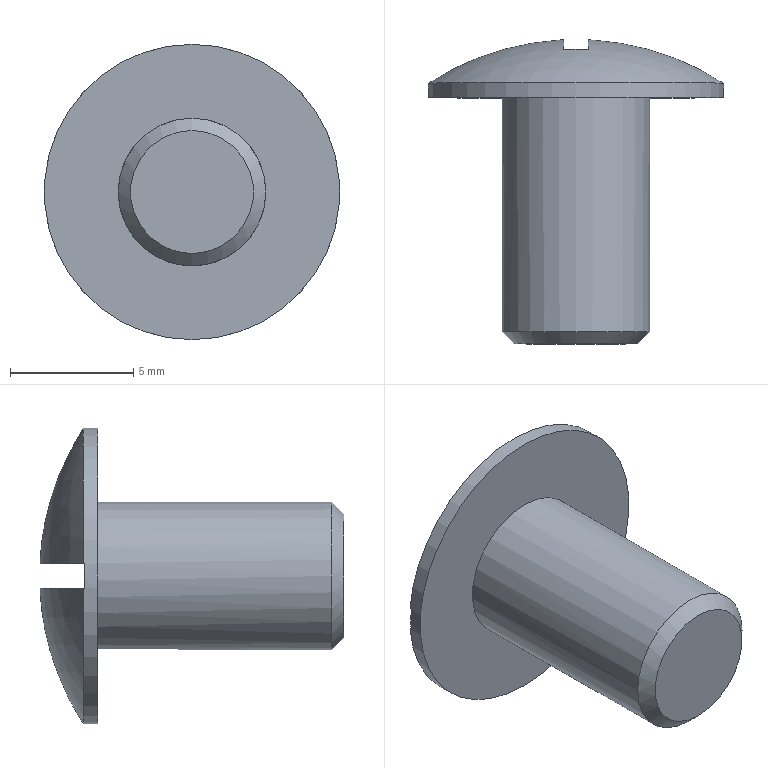Part | STEP file | PN_0016 | 1 solid | 22 faces | box 12 x 12.352 x 12 mm | volume 428.238 mm3 | plane 13 | cylinder 6 | sphere 2 | cone 1 | commonest cylinder face diameters 0.4 x4 6 x1 12 x1